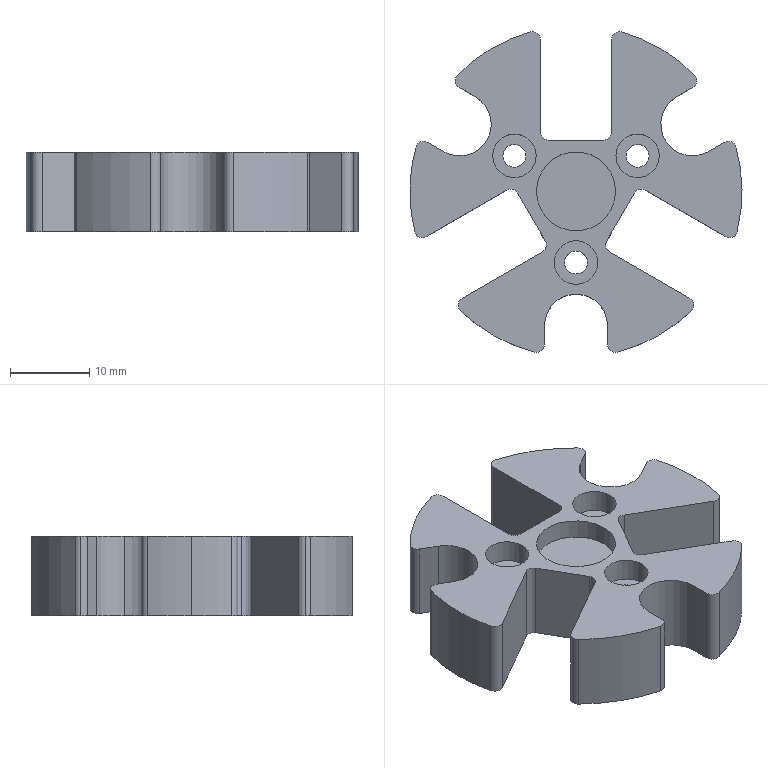Part | SolidWorks | features CirPattern 3, ICE 3, Fillet 2, Extrusion 1, HoleWzd 1 | 1 solid | 67 faces | box 42 x 40.594 x 10 mm | volume 7724 mm3 | cylinder 46 | plane 21 | commonest cylinder face diameters 2 x21 42 x7 2.9 x6 5.5 x6 8 x4 10 x2